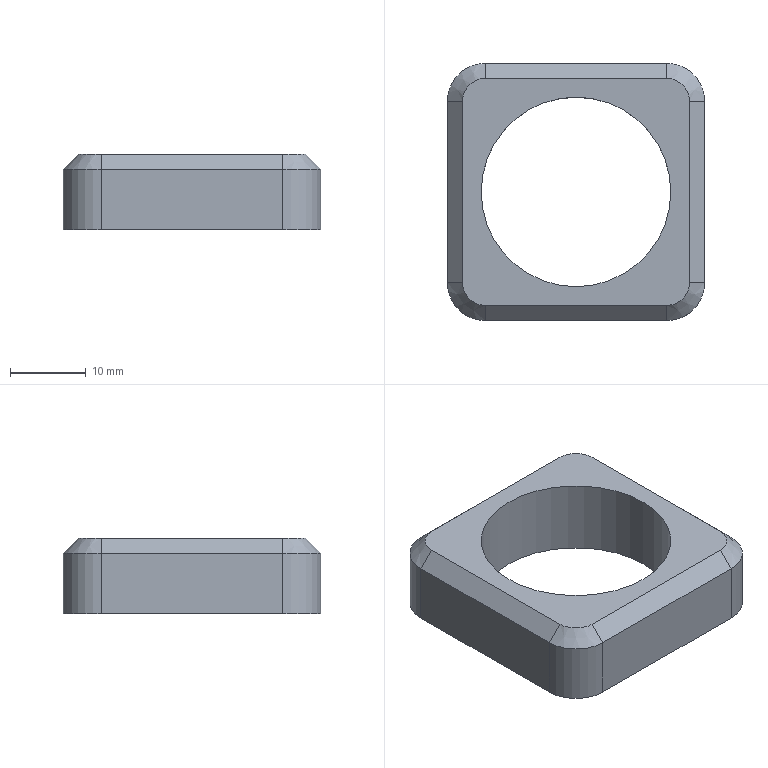Part | STEP file | Sheet34 | 1 solid | 19 faces | box 34 x 34 x 10 mm | volume 6171 mm3 | plane 10 | cylinder 5 | cone 4 | commonest cylinder face diameters 10 x4 25.05 x1
STEP:
#1=CARTESIAN_POINT('',(0.,0.,0.));
#2=DIRECTION('',(0.,0.,1.));
#3=DIRECTION('',(1.,0.,0.));
#4=AXIS2_PLACEMENT_3D('',#1,#2,#3);
#5=CARTESIAN_POINT('',(29.525,-17.,-7.));
#6=VERTEX_POINT('',#5);
#7=CARTESIAN_POINT('',(17.,-17.,-7.));
#8=DIRECTION('',(0.,0.,1.));
#9=DIRECTION('',(-1.,0.,0.));
#10=AXIS2_PLACEMENT_3D('',#7,#8,#9);
#11=CIRCLE('',#10,12.525);
#12=CARTESIAN_POINT('',(17.,-17.,3.));
#13=DIRECTION('',(0.,0.,-1.));
#14=DIRECTION('',(-1.,0.,0.));
#15=AXIS2_PLACEMENT_3D('',#12,#13,#14);
#16=CYLINDRICAL_SURFACE('',#15,12.525);
#17=CARTESIAN_POINT('',(12.566,10.));
#18=DIRECTION('',(-1.,0.));
#19=VECTOR('',#18,1.);
#20=LINE('',#17,#19);
#21=(GEOMETRIC_REPRESENTATION_CONTEXT(2)PARAMETRIC_REPRESENTATION_CONTEXT()REPRESENTATION_CONTEXT('',''));
#22=DEFINITIONAL_REPRESENTATION('',(#20),#21);
#23=PCURVE('',#16,#22);
#24=CARTESIAN_POINT('',(17.,-17.,-7.));
#25=DIRECTION('',(0.,0.,1.));
#26=DIRECTION('',(1.,0.,0.));
#27=AXIS2_PLACEMENT_3D('',#24,#25,#26);
#28=PLANE('',#27);
#29=CARTESIAN_POINT('',(0.,0.));
#30=DIRECTION('',(-1.,0.));
#31=AXIS2_PLACEMENT_2D('',#29,#30);
#32=CIRCLE('',#31,12.525);
#33=(GEOMETRIC_REPRESENTATION_CONTEXT(2)PARAMETRIC_REPRESENTATION_CONTEXT()REPRESENTATION_CONTEXT('',''));
#34=DEFINITIONAL_REPRESENTATION('',(#32),#33);
#35=PCURVE('',#28,#34);
#36=SURFACE_CURVE('',#11,(#23,#35),.PCURVE_S1.);
#37=EDGE_CURVE('',#6,#6,#36,.T.);
#38=ORIENTED_EDGE('',*,*,#37,.T.);
#39=CARTESIAN_POINT('',(29.525,-17.,3.));
#40=VERTEX_POINT('',#39);
#41=CARTESIAN_POINT('',(29.525,-17.,3.));
#42=CARTESIAN_POINT('',(29.525,-17.,-7.));
#43=B_SPLINE_CURVE_WITH_KNOTS('',1,(#41,#42),.UNSPECIFIED.,.F.,.F.,(2,2),(0.,10.),.PIECEWISE_BEZIER_KNOTS.);
#44=CARTESIAN_POINT('',(3.142,0.));
#45=DIRECTION('',(0.,1.));
#46=VECTOR('',#45,1.);
#47=LINE('',#44,#46);
#48=(GEOMETRIC_REPRESENTATION_CONTEXT(2)PARAMETRIC_REPRESENTATION_CONTEXT()REPRESENTATION_CONTEXT('',''));
#49=DEFINITIONAL_REPRESENTATION('',(#47),#48);
#50=PCURVE('',#16,#49);
#51=CARTESIAN_POINT('',(9.425,0.));
#52=DIRECTION('',(0.,1.));
#53=VECTOR('',#52,1.);
#54=LINE('',#51,#53);
#55=(GEOMETRIC_REPRESENTATION_CONTEXT(2)PARAMETRIC_REPRESENTATION_CONTEXT()REPRESENTATION_CONTEXT('',''));
#56=DEFINITIONAL_REPRESENTATION('',(#54),#55);
#57=PCURVE('',#16,#56);
#58=SEAM_CURVE('',#43,(#50,#57),.PCURVE_S1.);
#59=EDGE_CURVE('',#40,#6,#58,.T.);
#60=ORIENTED_EDGE('',*,*,#59,.F.);
#61=CARTESIAN_POINT('',(17.,-17.,3.));
#62=DIRECTION('',(0.,0.,-1.));
#63=DIRECTION('',(-1.,0.,0.));
#64=AXIS2_PLACEMENT_3D('',#61,#62,#63);
#65=CIRCLE('',#64,12.525);
#66=CARTESIAN_POINT('',(0.,0.));
#67=DIRECTION('',(1.,0.));
#68=VECTOR('',#67,1.);
#69=LINE('',#66,#68);
#70=(GEOMETRIC_REPRESENTATION_CONTEXT(2)PARAMETRIC_REPRESENTATION_CONTEXT()REPRESENTATION_CONTEXT('',''));
#71=DEFINITIONAL_REPRESENTATION('',(#69),#70);
#72=PCURVE('',#16,#71);
#73=CARTESIAN_POINT('',(17.,-17.,3.));
#74=DIRECTION('',(0.,0.,1.));
#75=DIRECTION('',(1.,0.,0.));
#76=AXIS2_PLACEMENT_3D('',#73,#74,#75);
#77=PLANE('',#76);
#78=CARTESIAN_POINT('',(-12.525,0.));
#79=CARTESIAN_POINT('',(-12.525,21.694));
#80=CARTESIAN_POINT('',(6.263,10.847));
#81=CARTESIAN_POINT('',(25.05,0.));
#82=CARTESIAN_POINT('',(6.263,-10.847));
#83=CARTESIAN_POINT('',(-12.525,-21.694));
#84=CARTESIAN_POINT('',(-12.525,0.));
#85=(BOUNDED_CURVE()B_SPLINE_CURVE(2,(#78,#79,#80,#81,#82,#83,#84),.UNSPECIFIED.,.T.,.F.)B_SPLINE_CURVE_WITH_KNOTS((1,2,2,2,2,1),(-2.094,0.,2.094,4.189,6.283,8.378),.UNSPECIFIED.)CURVE()GEOMETRIC_REPRESENTATION_ITEM()RATIONAL_B_SPLINE_CURVE((1.,0.5,1.,0.5,1.,0.5,1.))REPRESENTATION_ITEM(''));
#86=(GEOMETRIC_REPRESENTATION_CONTEXT(2)PARAMETRIC_REPRESENTATION_CONTEXT()REPRESENTATION_CONTEXT('',''));
#87=DEFINITIONAL_REPRESENTATION('',(#85),#86);
#88=PCURVE('',#77,#87);
#89=SURFACE_CURVE('',#65,(#72,#88),.PCURVE_S1.);
#90=EDGE_CURVE('',#40,#40,#89,.T.);
#91=ORIENTED_EDGE('',*,*,#90,.T.);
#92=ORIENTED_EDGE('',*,*,#59,.T.);
#93=EDGE_LOOP('',(#38,#60,#91,#92));
#94=FACE_BOUND('',#93,.F.);
#95=ADVANCED_FACE('',(#94),#16,.F.);
#96=CARTESIAN_POINT('',(29.,0.,1.));
#97=VERTEX_POINT('',#96);
#98=CARTESIAN_POINT('',(29.,-2.,3.));
#99=VERTEX_POINT('',#98);
#100=CARTESIAN_POINT('',(29.,0.,1.));
#101=DIRECTION('',(0.,-0.7071,0.7071));
#102=VECTOR('',#101,1.);
#103=LINE('',#100,#102);
#104=CARTESIAN_POINT('',(29.,-5.,2.));
#105=DIRECTION('',(0.,0.,-1.));
#106=DIRECTION('',(1.,0.,0.));
#107=AXIS2_PLACEMENT_3D('',#104,#105,#106);
#108=CONICAL_SURFACE('',#107,4.,0.7854);
#109=CARTESIAN_POINT('',(4.712,1.));
#110=DIRECTION('',(0.,-1.));
#111=VECTOR('',#110,1.);
#112=LINE('',#109,#111);
#113=(GEOMETRIC_REPRESENTATION_CONTEXT(2)PARAMETRIC_REPRESENTATION_CONTEXT()REPRESENTATION_CONTEXT('',''));
#114=DEFINITIONAL_REPRESENTATION('',(#112),#113);
#115=PCURVE('',#108,#114);
#116=CARTESIAN_POINT('',(23.,-1.,2.));
#117=DIRECTION('',(0.,0.7071,0.7071));
#118=DIRECTION('',(1.,0.,0.));
#119=AXIS2_PLACEMENT_3D('',#116,#117,#118);
#120=PLANE('',#119);
#121=CARTESIAN_POINT('',(6.,1.414));
#122=DIRECTION('',(0.,-1.));
#123=VECTOR('',#122,1.);
#124=LINE('',#121,#123);
#125=(GEOMETRIC_REPRESENTATION_CONTEXT(2)PARAMETRIC_REPRESENTATION_CONTEXT()REPRESENTATION_CONTEXT('',''));
#126=DEFINITIONAL_REPRESENTATION('',(#124),#125);
#127=PCURVE('',#120,#126);
#128=SURFACE_CURVE('',#103,(#115,#127),.PCURVE_S1.);
#129=EDGE_CURVE('',#97,#99,#128,.T.);
#130=ORIENTED_EDGE('',*,*,#129,.T.);
#131=CARTESIAN_POINT('',(32.,-5.,3.));
#132=VERTEX_POINT('',#131);
#133=CARTESIAN_POINT('',(29.,-5.,3.));
#134=DIRECTION('',(0.,0.,-1.));
#135=DIRECTION('',(1.,0.,0.));
#136=AXIS2_PLACEMENT_3D('',#133,#134,#135);
#137=CIRCLE('',#136,3.);
#138=CARTESIAN_POINT('',(0.,-1.));
#139=DIRECTION('',(1.,0.));
#140=VECTOR('',#139,1.);
#141=LINE('',#138,#140);
#142=(GEOMETRIC_REPRESENTATION_CONTEXT(2)PARAMETRIC_REPRESENTATION_CONTEXT()REPRESENTATION_CONTEXT('',''));
#143=DEFINITIONAL_REPRESENTATION('',(#141),#142);
#144=PCURVE('',#108,#143);
#145=CARTESIAN_POINT('',(15.,12.));
#146=CARTESIAN_POINT('',(15.,6.804));
#147=CARTESIAN_POINT('',(10.5,9.402));
#148=CARTESIAN_POINT('',(6.,12.));
#149=CARTESIAN_POINT('',(10.5,14.598));
#150=CARTESIAN_POINT('',(15.,17.196));
#151=CARTESIAN_POINT('',(15.,12.));
#152=(BOUNDED_CURVE()B_SPLINE_CURVE(2,(#145,#146,#147,#148,#149,#150,#151),.UNSPECIFIED.,.T.,.F.)B_SPLINE_CURVE_WITH_KNOTS((1,2,2,2,2,1),(-2.094,0.,2.094,4.189,6.283,8.378),.UNSPECIFIED.)CURVE()GEOMETRIC_REPRESENTATION_ITEM()RATIONAL_B_SPLINE_CURVE((1.,0.5,1.,0.5,1.,0.5,1.))REPRESENTATION_ITEM(''));
#153=(GEOMETRIC_REPRESENTATION_CONTEXT(2)PARAMETRIC_REPRESENTATION_CONTEXT()REPRESENTATION_CONTEXT('',''));
#154=DEFINITIONAL_REPRESENTATION('',(#152),#153);
#155=PCURVE('',#77,#154);
#156=SURFACE_CURVE('',#137,(#144,#155),.PCURVE_S1.);
#157=EDGE_CURVE('',#99,#132,#156,.T.);
#158=ORIENTED_EDGE('',*,*,#157,.T.);
#159=CARTESIAN_POINT('',(34.,-5.,1.));
#160=VERTEX_POINT('',#159);
#161=CARTESIAN_POINT('',(32.,-5.,3.));
#162=DIRECTION('',(0.7071,0.,-0.7071));
#163=VECTOR('',#162,1.);
#164=LINE('',#161,#163);
#165=CARTESIAN_POINT('',(6.283,-1.));
#166=DIRECTION('',(0.,1.));
#167=VECTOR('',#166,1.);
#168=LINE('',#165,#167);
#169=(GEOMETRIC_REPRESENTATION_CONTEXT(2)PARAMETRIC_REPRESENTATION_CONTEXT()REPRESENTATION_CONTEXT('',''));
#170=DEFINITIONAL_REPRESENTATION('',(#168),#169);
#171=PCURVE('',#108,#170);
#172=CARTESIAN_POINT('',(33.,-23.,2.));
#173=DIRECTION('',(0.7071,0.,0.7071));
#174=DIRECTION('',(0.7071,0.,-0.7071));
#175=AXIS2_PLACEMENT_3D('',#172,#173,#174);
#176=PLANE('',#175);
#177=CARTESIAN_POINT('',(-1.414,18.));
#178=DIRECTION('',(1.,0.));
#179=VECTOR('',#178,1.);
#180=LINE('',#177,#179);
#181=(GEOMETRIC_REPRESENTATION_CONTEXT(2)PARAMETRIC_REPRESENTATION_CONTEXT()REPRESENTATION_CONTEXT('',''));
#182=DEFINITIONAL_REPRESENTATION('',(#180),#181);
#183=PCURVE('',#176,#182);
#184=SURFACE_CURVE('',#164,(#171,#183),.PCURVE_S1.);
#185=EDGE_CURVE('',#132,#160,#184,.T.);
#186=ORIENTED_EDGE('',*,*,#185,.T.);
#187=CARTESIAN_POINT('',(29.,-5.,1.));
#188=DIRECTION('',(0.,0.,1.));
#189=DIRECTION('',(1.,0.,0.));
#190=AXIS2_PLACEMENT_3D('',#187,#188,#189);
#191=CIRCLE('',#190,5.);
#192=CARTESIAN_POINT('',(6.283,1.));
#193=DIRECTION('',(-1.,0.));
#194=VECTOR('',#193,1.);
#195=LINE('',#192,#194);
#196=(GEOMETRIC_REPRESENTATION_CONTEXT(2)PARAMETRIC_REPRESENTATION_CONTEXT()REPRESENTATION_CONTEXT('',''));
#197=DEFINITIONAL_REPRESENTATION('',(#195),#196);
#198=PCURVE('',#108,#197);
#199=CARTESIAN_POINT('',(29.,-5.,0.));
#200=DIRECTION('',(0.,0.,1.));
#201=DIRECTION('',(-1.,0.,0.));
#202=AXIS2_PLACEMENT_3D('',#199,#200,#201);
#203=CYLINDRICAL_SURFACE('',#202,5.);
#204=CARTESIAN_POINT('',(3.142,1.));
#205=DIRECTION('',(1.,0.));
#206=VECTOR('',#205,1.);
#207=LINE('',#204,#206);
#208=(GEOMETRIC_REPRESENTATION_CONTEXT(2)PARAMETRIC_REPRESENTATION_CONTEXT()REPRESENTATION_CONTEXT('',''));
#209=DEFINITIONAL_REPRESENTATION('',(#207),#208);
#210=PCURVE('',#203,#209);
#211=SURFACE_CURVE('',#191,(#198,#210),.PCURVE_S1.);
#212=EDGE_CURVE('',#160,#97,#211,.T.);
#213=ORIENTED_EDGE('',*,*,#212,.T.);
#214=EDGE_LOOP('',(#130,#158,#186,#213));
#215=FACE_BOUND('',#214,.T.);
#216=ADVANCED_FACE('',(#215),#108,.T.);
#217=CARTESIAN_POINT('',(5.,0.,1.));
#218=VERTEX_POINT('',#217);
#219=CARTESIAN_POINT('',(5.,-2.,3.));
#220=VERTEX_POINT('',#219);
#221=CARTESIAN_POINT('',(5.,0.,1.));
#222=DIRECTION('',(0.,-0.7071,0.7071));
#223=VECTOR('',#222,1.);
#224=LINE('',#221,#223);
#225=CARTESIAN_POINT('',(-18.,1.414));
#226=DIRECTION('',(0.,-1.));
#227=VECTOR('',#226,1.);
#228=LINE('',#225,#227);
#229=(GEOMETRIC_REPRESENTATION_CONTEXT(2)PARAMETRIC_REPRESENTATION_CONTEXT()REPRESENTATION_CONTEXT('',''));
#230=DEFINITIONAL_REPRESENTATION('',(#228),#229);
#231=PCURVE('',#120,#230);
#232=CARTESIAN_POINT('',(5.,-5.,2.));
#233=DIRECTION('',(0.,0.,-1.));
#234=DIRECTION('',(0.,1.,0.));
#235=AXIS2_PLACEMENT_3D('',#232,#233,#234);
#236=CONICAL_SURFACE('',#235,4.,0.7854);
#237=CARTESIAN_POINT('',(6.283,1.));
#238=DIRECTION('',(0.,-1.));
#239=VECTOR('',#238,1.);
#240=LINE('',#237,#239);
#241=(GEOMETRIC_REPRESENTATION_CONTEXT(2)PARAMETRIC_REPRESENTATION_CONTEXT()REPRESENTATION_CONTEXT('',''));
#242=DEFINITIONAL_REPRESENTATION('',(#240),#241);
#243=PCURVE('',#236,#242);
#244=SURFACE_CURVE('',#224,(#231,#243),.PCURVE_S1.);
#245=EDGE_CURVE('',#218,#220,#244,.T.);
#246=ORIENTED_EDGE('',*,*,#245,.T.);
#247=CARTESIAN_POINT('',(23.,-2.,3.));
#248=DIRECTION('',(1.,0.,0.));
#249=VECTOR('',#248,1.);
#250=LINE('',#247,#249);
#251=CARTESIAN_POINT('',(0.,-1.414));
#252=DIRECTION('',(1.,0.));
#253=VECTOR('',#252,1.);
#254=LINE('',#251,#253);
#255=(GEOMETRIC_REPRESENTATION_CONTEXT(2)PARAMETRIC_REPRESENTATION_CONTEXT()REPRESENTATION_CONTEXT('',''));
#256=DEFINITIONAL_REPRESENTATION('',(#254),#255);
#257=PCURVE('',#120,#256);
#258=CARTESIAN_POINT('',(6.,15.));
#259=DIRECTION('',(1.,0.));
#260=VECTOR('',#259,1.);
#261=LINE('',#258,#260);
#262=(GEOMETRIC_REPRESENTATION_CONTEXT(2)PARAMETRIC_REPRESENTATION_CONTEXT()REPRESENTATION_CONTEXT('',''));
#263=DEFINITIONAL_REPRESENTATION('',(#261),#262);
#264=PCURVE('',#77,#263);
#265=SURFACE_CURVE('',#250,(#257,#264),.PCURVE_S1.);
#266=EDGE_CURVE('',#220,#99,#265,.T.);
#267=ORIENTED_EDGE('',*,*,#266,.T.);
#268=ORIENTED_EDGE('',*,*,#129,.F.);
#269=CARTESIAN_POINT('',(23.,0.,1.));
#270=DIRECTION('',(-1.,0.,0.));
#271=VECTOR('',#270,1.);
#272=LINE('',#269,#271);
#273=CARTESIAN_POINT('',(0.,1.414));
#274=DIRECTION('',(-1.,0.));
#275=VECTOR('',#274,1.);
#276=LINE('',#273,#275);
#277=(GEOMETRIC_REPRESENTATION_CONTEXT(2)PARAMETRIC_REPRESENTATION_CONTEXT()REPRESENTATION_CONTEXT('',''));
#278=DEFINITIONAL_REPRESENTATION('',(#276),#277);
#279=PCURVE('',#120,#278);
#280=CARTESIAN_POINT('',(29.,0.,0.));
#281=DIRECTION('',(0.,1.,0.));
#282=DIRECTION('',(-1.,0.,0.));
#283=AXIS2_PLACEMENT_3D('',#280,#281,#282);
#284=PLANE('',#283);
#285=CARTESIAN_POINT('',(6.,1.));
#286=DIRECTION('',(1.,0.));
#287=VECTOR('',#286,1.);
#288=LINE('',#285,#287);
#289=(GEOMETRIC_REPRESENTATION_CONTEXT(2)PARAMETRIC_REPRESENTATION_CONTEXT()REPRESENTATION_CONTEXT('',''));
#290=DEFINITIONAL_REPRESENTATION('',(#288),#289);
#291=PCURVE('',#284,#290);
#292=SURFACE_CURVE('',#272,(#279,#291),.PCURVE_S1.);
#293=EDGE_CURVE('',#97,#218,#292,.T.);
#294=ORIENTED_EDGE('',*,*,#293,.T.);
#295=EDGE_LOOP('',(#246,#267,#268,#294));
#296=FACE_BOUND('',#295,.T.);
#297=ADVANCED_FACE('',(#296),#120,.T.);
#298=CARTESIAN_POINT('',(0.,-5.,1.));
#299=VERTEX_POINT('',#298);
#300=CARTESIAN_POINT('',(2.,-5.,3.));
#301=VERTEX_POINT('',#300);
#302=CARTESIAN_POINT('',(0.,-5.,1.));
#303=DIRECTION('',(0.7071,0.,0.7071));
#304=VECTOR('',#303,1.);
#305=LINE('',#302,#304);
#306=CARTESIAN_POINT('',(4.712,1.));
#307=DIRECTION('',(0.,-1.));
#308=VECTOR('',#307,1.);
#309=LINE('',#306,#308);
#310=(GEOMETRIC_REPRESENTATION_CONTEXT(2)PARAMETRIC_REPRESENTATION_CONTEXT()REPRESENTATION_CONTEXT('',''));
#311=DEFINITIONAL_REPRESENTATION('',(#309),#310);
#312=PCURVE('',#236,#311);
#313=CARTESIAN_POINT('',(1.,-11.,2.));
#314=DIRECTION('',(-0.7071,0.,0.7071));
#315=DIRECTION('',(0.7071,0.,0.7071));
#316=AXIS2_PLACEMENT_3D('',#313,#314,#315);
#317=PLANE('',#316);
#318=CARTESIAN_POINT('',(-1.414,6.));
#319=DIRECTION('',(1.,0.));
#320=VECTOR('',#319,1.);
#321=LINE('',#318,#320);
#322=(GEOMETRIC_REPRESENTATION_CONTEXT(2)PARAMETRIC_REPRESENTATION_CONTEXT()REPRESENTATION_CONTEXT('',''));
#323=DEFINITIONAL_REPRESENTATION('',(#321),#322);
#324=PCURVE('',#317,#323);
#325=SURFACE_CURVE('',#305,(#312,#324),.PCURVE_S1.);
#326=EDGE_CURVE('',#299,#301,#325,.T.);
#327=ORIENTED_EDGE('',*,*,#326,.T.);
#328=CARTESIAN_POINT('',(5.,-5.,3.));
#329=DIRECTION('',(0.,0.,-1.));
#330=DIRECTION('',(0.,1.,0.));
#331=AXIS2_PLACEMENT_3D('',#328,#329,#330);
#332=CIRCLE('',#331,3.);
#333=CARTESIAN_POINT('',(0.,-1.));
#334=DIRECTION('',(1.,0.));
#335=VECTOR('',#334,1.);
#336=LINE('',#333,#335);
#337=(GEOMETRIC_REPRESENTATION_CONTEXT(2)PARAMETRIC_REPRESENTATION_CONTEXT()REPRESENTATION_CONTEXT('',''));
#338=DEFINITIONAL_REPRESENTATION('',(#336),#337);
#339=PCURVE('',#236,#338);
#340=CARTESIAN_POINT('',(-12.,15.));
#341=CARTESIAN_POINT('',(-6.804,15.));
#342=CARTESIAN_POINT('',(-9.402,10.5));
#343=CARTESIAN_POINT('',(-12.,6.));
#344=CARTESIAN_POINT('',(-14.598,10.5));
#345=CARTESIAN_POINT('',(-17.196,15.));
#346=CARTESIAN_POINT('',(-12.,15.));
#347=(BOUNDED_CURVE()B_SPLINE_CURVE(2,(#340,#341,#342,#343,#344,#345,#346),.UNSPECIFIED.,.T.,.F.)B_SPLINE_CURVE_WITH_KNOTS((1,2,2,2,2,1),(-2.094,0.,2.094,4.189,6.283,8.378),.UNSPECIFIED.)CURVE()GEOMETRIC_REPRESENTATION_ITEM()RATIONAL_B_SPLINE_CURVE((1.,0.5,1.,0.5,1.,0.5,1.))REPRESENTATION_ITEM(''));
#348=(GEOMETRIC_REPRESENTATION_CONTEXT(2)PARAMETRIC_REPRESENTATION_CONTEXT()REPRESENTATION_CONTEXT('',''));
#349=DEFINITIONAL_REPRESENTATION('',(#347),#348);
#350=PCURVE('',#77,#349);
#351=SURFACE_CURVE('',#332,(#339,#350),.PCURVE_S1.);
#352=EDGE_CURVE('',#301,#220,#351,.T.);
#353=ORIENTED_EDGE('',*,*,#352,.T.);
#354=ORIENTED_EDGE('',*,*,#245,.F.);
#355=CARTESIAN_POINT('',(5.,-5.,1.));
#356=DIRECTION('',(0.,0.,1.));
#357=DIRECTION('',(0.,1.,0.));
#358=AXIS2_PLACEMENT_3D('',#355,#356,#357);
#359=CIRCLE('',#358,5.);
#360=CARTESIAN_POINT('',(6.283,1.));
#361=DIRECTION('',(-1.,0.));
#362=VECTOR('',#361,1.);
#363=LINE('',#360,#362);
#364=(GEOMETRIC_REPRESENTATION_CONTEXT(2)PARAMETRIC_REPRESENTATION_CONTEXT()REPRESENTATION_CONTEXT('',''));
#365=DEFINITIONAL_REPRESENTATION('',(#363),#364);
#366=PCURVE('',#236,#365);
#367=CARTESIAN_POINT('',(5.,-5.,0.));
#368=DIRECTION('',(0.,0.,1.));
#369=DIRECTION('',(0.,-1.,0.));
#370=AXIS2_PLACEMENT_3D('',#367,#368,#369);
#371=CYLINDRICAL_SURFACE('',#370,5.);
#372=CARTESIAN_POINT('',(3.142,1.));
#373=DIRECTION('',(1.,0.));
#374=VECTOR('',#373,1.);
#375=LINE('',#372,#374);
#376=(GEOMETRIC_REPRESENTATION_CONTEXT(2)PARAMETRIC_REPRESENTATION_CONTEXT()REPRESENTATION_CONTEXT('',''));
#377=DEFINITIONAL_REPRESENTATION('',(#375),#376);
#378=PCURVE('',#371,#377);
#379=SURFACE_CURVE('',#359,(#366,#378),.PCURVE_S1.);
#380=EDGE_CURVE('',#218,#299,#379,.T.);
#381=ORIENTED_EDGE('',*,*,#380,.T.);
#382=EDGE_LOOP('',(#327,#353,#354,#381));
#383=FACE_BOUND('',#382,.T.);
#384=ADVANCED_FACE('',(#383),#236,.T.);
#385=CARTESIAN_POINT('',(0.,-29.,1.));
#386=VERTEX_POINT('',#385);
#387=CARTESIAN_POINT('',(2.,-29.,3.));
#388=VERTEX_POINT('',#387);
#389=CARTESIAN_POINT('',(0.,-29.,1.));
#390=DIRECTION('',(0.7071,0.,0.7071));
#391=VECTOR('',#390,1.);
#392=LINE('',#389,#391);
#393=CARTESIAN_POINT('',(-1.414,-18.));
#394=DIRECTION('',(1.,0.));
#395=VECTOR('',#394,1.);
#396=LINE('',#393,#395);
#397=(GEOMETRIC_REPRESENTATION_CONTEXT(2)PARAMETRIC_REPRESENTATION_CONTEXT()REPRESENTATION_CONTEXT('',''));
#398=DEFINITIONAL_REPRESENTATION('',(#396),#397);
#399=PCURVE('',#317,#398);
#400=CARTESIAN_POINT('',(5.,-29.,2.));
#401=DIRECTION('',(0.,0.,-1.));
#402=DIRECTION('',(-1.,0.,0.));
#403=AXIS2_PLACEMENT_3D('',#400,#401,#402);
#404=CONICAL_SURFACE('',#403,4.,0.7854);
#405=CARTESIAN_POINT('',(6.283,1.));
#406=DIRECTION('',(0.,-1.));
#407=VECTOR('',#406,1.);
#408=LINE('',#405,#407);
#409=(GEOMETRIC_REPRESENTATION_CONTEXT(2)PARAMETRIC_REPRESENTATION_CONTEXT()REPRESENTATION_CONTEXT('',''));
#410=DEFINITIONAL_REPRESENTATION('',(#408),#409);
#411=PCURVE('',#404,#410);
#412=SURFACE_CURVE('',#392,(#399,#411),.PCURVE_S1.);
#413=EDGE_CURVE('',#386,#388,#412,.T.);
#414=ORIENTED_EDGE('',*,*,#413,.T.);
#415=CARTESIAN_POINT('',(2.,-11.,3.));
#416=DIRECTION('',(0.,1.,0.));
#417=VECTOR('',#416,1.);
#418=LINE('',#415,#417);
#419=CARTESIAN_POINT('',(1.414,0.));
#420=DIRECTION('',(0.,1.));
#421=VECTOR('',#420,1.);
#422=LINE('',#419,#421);
#423=(GEOMETRIC_REPRESENTATION_CONTEXT(2)PARAMETRIC_REPRESENTATION_CONTEXT()REPRESENTATION_CONTEXT('',''));
#424=DEFINITIONAL_REPRESENTATION('',(#422),#423);
#425=PCURVE('',#317,#424);
#426=CARTESIAN_POINT('',(-15.,6.));
#427=DIRECTION('',(0.,1.));
#428=VECTOR('',#427,1.);
#429=LINE('',#426,#428);
#430=(GEOMETRIC_REPRESENTATION_CONTEXT(2)PARAMETRIC_REPRESENTATION_CONTEXT()REPRESENTATION_CONTEXT('',''));
#431=DEFINITIONAL_REPRESENTATION('',(#429),#430);
#432=PCURVE('',#77,#431);
#433=SURFACE_CURVE('',#418,(#425,#432),.PCURVE_S1.);
#434=EDGE_CURVE('',#388,#301,#433,.T.);
#435=ORIENTED_EDGE('',*,*,#434,.T.);
#436=ORIENTED_EDGE('',*,*,#326,.F.);
#437=CARTESIAN_POINT('',(0.,-11.,1.));
#438=DIRECTION('',(0.,-1.,0.));
#439=VECTOR('',#438,1.);
#440=LINE('',#437,#439);
#441=CARTESIAN_POINT('',(-1.414,0.));
#442=DIRECTION('',(0.,-1.));
#443=VECTOR('',#442,1.);
#444=LINE('',#441,#443);
#445=(GEOMETRIC_REPRESENTATION_CONTEXT(2)PARAMETRIC_REPRESENTATION_CONTEXT()REPRESENTATION_CONTEXT('',''));
#446=DEFINITIONAL_REPRESENTATION('',(#444),#445);
#447=PCURVE('',#317,#446);
#448=CARTESIAN_POINT('',(0.,-5.,0.));
#449=DIRECTION('',(-1.,0.,0.));
#450=DIRECTION('',(0.,-1.,0.));
#451=AXIS2_PLACEMENT_3D('',#448,#449,#450);
#452=PLANE('',#451);
#453=CARTESIAN_POINT('',(6.,1.));
#454=DIRECTION('',(1.,0.));
#455=VECTOR('',#454,1.);
#456=LINE('',#453,#455);
#457=(GEOMETRIC_REPRESENTATION_CONTEXT(2)PARAMETRIC_REPRESENTATION_CONTEXT()REPRESENTATION_CONTEXT('',''));
#458=DEFINITIONAL_REPRESENTATION('',(#456),#457);
#459=PCURVE('',#452,#458);
#460=SURFACE_CURVE('',#440,(#447,#459),.PCURVE_S1.);
#461=EDGE_CURVE('',#299,#386,#460,.T.);
#462=ORIENTED_EDGE('',*,*,#461,.T.);
#463=EDGE_LOOP('',(#414,#435,#436,#462));
#464=FACE_BOUND('',#463,.T.);
#465=ADVANCED_FACE('',(#464),#317,.T.);
#466=CARTESIAN_POINT('',(5.,-34.,1.));
#467=VERTEX_POINT('',#466);
#468=CARTESIAN_POINT('',(5.,-32.,3.));
#469=VERTEX_POINT('',#468);
#470=CARTESIAN_POINT('',(5.,-34.,1.));
#471=DIRECTION('',(0.,0.7071,0.7071));
#472=VECTOR('',#471,1.);
#473=LINE('',#470,#472);
#474=CARTESIAN_POINT('',(4.712,1.));
#475=DIRECTION('',(0.,-1.));
#476=VECTOR('',#475,1.);
#477=LINE('',#474,#476);
#478=(GEOMETRIC_REPRESENTATION_CONTEXT(2)PARAMETRIC_REPRESENTATION_CONTEXT()REPRESENTATION_CONTEXT('',''));
#479=DEFINITIONAL_REPRESENTATION('',(#477),#478);
#480=PCURVE('',#404,#479);
#481=CARTESIAN_POINT('',(11.,-33.,2.));
#482=DIRECTION('',(0.,-0.7071,0.7071));
#483=DIRECTION('',(1.,0.,0.));
#484=AXIS2_PLACEMENT_3D('',#481,#482,#483);
#485=PLANE('',#484);
#486=CARTESIAN_POINT('',(-6.,-1.414));
#487=DIRECTION('',(0.,1.));
#488=VECTOR('',#487,1.);
#489=LINE('',#486,#488);
#490=(GEOMETRIC_REPRESENTATION_CONTEXT(2)PARAMETRIC_REPRESENTATION_CONTEXT()REPRESENTATION_CONTEXT('',''));
#491=DEFINITIONAL_REPRESENTATION('',(#489),#490);
#492=PCURVE('',#485,#491);
#493=SURFACE_CURVE('',#473,(#480,#492),.PCURVE_S1.);
#494=EDGE_CURVE('',#467,#469,#493,.T.);
#495=ORIENTED_EDGE('',*,*,#494,.T.);
#496=CARTESIAN_POINT('',(5.,-29.,3.));
#497=DIRECTION('',(0.,0.,-1.));
#498=DIRECTION('',(-1.,0.,0.));
#499=AXIS2_PLACEMENT_3D('',#496,#497,#498);
#500=CIRCLE('',#499,3.);
#501=CARTESIAN_POINT('',(0.,-1.));
#502=DIRECTION('',(1.,0.));
#503=VECTOR('',#502,1.);
#504=LINE('',#501,#503);
#505=(GEOMETRIC_REPRESENTATION_CONTEXT(2)PARAMETRIC_REPRESENTATION_CONTEXT()REPRESENTATION_CONTEXT('',''));
#506=DEFINITIONAL_REPRESENTATION('',(#504),#505);
#507=PCURVE('',#404,#506);
#508=CARTESIAN_POINT('',(-15.,-12.));
#509=CARTESIAN_POINT('',(-15.,-6.804));
#510=CARTESIAN_POINT('',(-10.5,-9.402));
#511=CARTESIAN_POINT('',(-6.,-12.));
#512=CARTESIAN_POINT('',(-10.5,-14.598));
#513=CARTESIAN_POINT('',(-15.,-17.196));
#514=CARTESIAN_POINT('',(-15.,-12.));
#515=(BOUNDED_CURVE()B_SPLINE_CURVE(2,(#508,#509,#510,#511,#512,#513,#514),.UNSPECIFIED.,.T.,.F.)B_SPLINE_CURVE_WITH_KNOTS((1,2,2,2,2,1),(-2.094,0.,2.094,4.189,6.283,8.378),.UNSPECIFIED.)CURVE()GEOMETRIC_REPRESENTATION_ITEM()RATIONAL_B_SPLINE_CURVE((1.,0.5,1.,0.5,1.,0.5,1.))REPRESENTATION_ITEM(''));
#516=(GEOMETRIC_REPRESENTATION_CONTEXT(2)PARAMETRIC_REPRESENTATION_CONTEXT()REPRESENTATION_CONTEXT('',''));
#517=DEFINITIONAL_REPRESENTATION('',(#515),#516);
#518=PCURVE('',#77,#517);
#519=SURFACE_CURVE('',#500,(#507,#518),.PCURVE_S1.);
#520=EDGE_CURVE('',#469,#388,#519,.T.);
#521=ORIENTED_EDGE('',*,*,#520,.T.);
#522=ORIENTED_EDGE('',*,*,#413,.F.);
#523=CARTESIAN_POINT('',(5.,-29.,1.));
#524=DIRECTION('',(0.,0.,1.));
#525=DIRECTION('',(-1.,0.,0.));
#526=AXIS2_PLACEMENT_3D('',#523,#524,#525);
#527=CIRCLE('',#526,5.);
#528=CARTESIAN_POINT('',(6.283,1.));
#529=DIRECTION('',(-1.,0.));
#530=VECTOR('',#529,1.);
#531=LINE('',#528,#530);
#532=(GEOMETRIC_REPRESENTATION_CONTEXT(2)PARAMETRIC_REPRESENTATION_CONTEXT()REPRESENTATION_CONTEXT('',''));
#533=DEFINITIONAL_REPRESENTATION('',(#531),#532);
#534=PCURVE('',#404,#533);
#535=CARTESIAN_POINT('',(5.,-29.,0.));
#536=DIRECTION('',(0.,0.,1.));
#537=DIRECTION('',(1.,0.,0.));
#538=AXIS2_PLACEMENT_3D('',#535,#536,#537);
#539=CYLINDRICAL_SURFACE('',#538,5.);
#540=CARTESIAN_POINT('',(3.142,1.));
#541=DIRECTION('',(1.,0.));
#542=VECTOR('',#541,1.);
#543=LINE('',#540,#542);
#544=(GEOMETRIC_REPRESENTATION_CONTEXT(2)PARAMETRIC_REPRESENTATION_CONTEXT()REPRESENTATION_CONTEXT('',''));
#545=DEFINITIONAL_REPRESENTATION('',(#543),#544);
#546=PCURVE('',#539,#545);
#547=SURFACE_CURVE('',#527,(#534,#546),.PCURVE_S1.);
#548=EDGE_CURVE('',#386,#467,#547,.T.);
#549=ORIENTED_EDGE('',*,*,#548,.T.);
#550=EDGE_LOOP('',(#495,#521,#522,#549));
#551=FACE_BOUND('',#550,.T.);
#552=ADVANCED_FACE('',(#551),#404,.T.);
#553=CARTESIAN_POINT('',(29.,-34.,1.));
#554=VERTEX_POINT('',#553);
#555=CARTESIAN_POINT('',(29.,-32.,3.));
#556=VERTEX_POINT('',#555);
#557=CARTESIAN_POINT('',(29.,-34.,1.));
#558=DIRECTION('',(0.,0.7071,0.7071));
#559=VECTOR('',#558,1.);
#560=LINE('',#557,#559);
#561=CARTESIAN_POINT('',(18.,-1.414));
#562=DIRECTION('',(0.,1.));
#563=VECTOR('',#562,1.);
#564=LINE('',#561,#563);
#565=(GEOMETRIC_REPRESENTATION_CONTEXT(2)PARAMETRIC_REPRESENTATION_CONTEXT()REPRESENTATION_CONTEXT('',''));
#566=DEFINITIONAL_REPRESENTATION('',(#564),#565);
#567=PCURVE('',#485,#566);
#568=CARTESIAN_POINT('',(29.,-29.,2.));
#569=DIRECTION('',(0.,0.,-1.));
#570=DIRECTION('',(0.,-1.,0.));
#571=AXIS2_PLACEMENT_3D('',#568,#569,#570);
#572=CONICAL_SURFACE('',#571,4.,0.7854);
#573=CARTESIAN_POINT('',(6.283,1.));
#574=DIRECTION('',(0.,-1.));
#575=VECTOR('',#574,1.);
#576=LINE('',#573,#575);
#577=(GEOMETRIC_REPRESENTATION_CONTEXT(2)PARAMETRIC_REPRESENTATION_CONTEXT()REPRESENTATION_CONTEXT('',''));
#578=DEFINITIONAL_REPRESENTATION('',(#576),#577);
#579=PCURVE('',#572,#578);
#580=SURFACE_CURVE('',#560,(#567,#579),.PCURVE_S1.);
#581=EDGE_CURVE('',#554,#556,#580,.T.);
#582=ORIENTED_EDGE('',*,*,#581,.T.);
#583=CARTESIAN_POINT('',(11.,-32.,3.));
#584=DIRECTION('',(-1.,0.,0.));
#585=VECTOR('',#584,1.);
#586=LINE('',#583,#585);
#587=CARTESIAN_POINT('',(0.,1.414));
#588=DIRECTION('',(-1.,0.));
#589=VECTOR('',#588,1.);
#590=LINE('',#587,#589);
#591=(GEOMETRIC_REPRESENTATION_CONTEXT(2)PARAMETRIC_REPRESENTATION_CONTEXT()REPRESENTATION_CONTEXT('',''));
#592=DEFINITIONAL_REPRESENTATION('',(#590),#591);
#593=PCURVE('',#485,#592);
#594=CARTESIAN_POINT('',(-6.,-15.));
#595=DIRECTION('',(-1.,0.));
#596=VECTOR('',#595,1.);
#597=LINE('',#594,#596);
#598=(GEOMETRIC_REPRESENTATION_CONTEXT(2)PARAMETRIC_REPRESENTATION_CONTEXT()REPRESENTATION_CONTEXT('',''));
#599=DEFINITIONAL_REPRESENTATION('',(#597),#598);
#600=PCURVE('',#77,#599);
#601=SURFACE_CURVE('',#586,(#593,#600),.PCURVE_S1.);
#602=EDGE_CURVE('',#556,#469,#601,.T.);
#603=ORIENTED_EDGE('',*,*,#602,.T.);
#604=ORIENTED_EDGE('',*,*,#494,.F.);
#605=CARTESIAN_POINT('',(11.,-34.,1.));
#606=DIRECTION('',(1.,0.,0.));
#607=VECTOR('',#606,1.);
#608=LINE('',#605,#607);
#609=CARTESIAN_POINT('',(0.,-1.414));
#610=DIRECTION('',(1.,0.));
#611=VECTOR('',#610,1.);
#612=LINE('',#609,#611);
#613=(GEOMETRIC_REPRESENTATION_CONTEXT(2)PARAMETRIC_REPRESENTATION_CONTEXT()REPRESENTATION_CONTEXT('',''));
#614=DEFINITIONAL_REPRESENTATION('',(#612),#613);
#615=PCURVE('',#485,#614);
#616=CARTESIAN_POINT('',(5.,-34.,0.));
#617=DIRECTION('',(0.,-1.,0.));
#618=DIRECTION('',(1.,0.,0.));
#619=AXIS2_PLACEMENT_3D('',#616,#617,#618);
#620=PLANE('',#619);
#621=CARTESIAN_POINT('',(6.,1.));
#622=DIRECTION('',(1.,0.));
#623=VECTOR('',#622,1.);
#624=LINE('',#621,#623);
#625=(GEOMETRIC_REPRESENTATION_CONTEXT(2)PARAMETRIC_REPRESENTATION_CONTEXT()REPRESENTATION_CONTEXT('',''));
#626=DEFINITIONAL_REPRESENTATION('',(#624),#625);
#627=PCURVE('',#620,#626);
#628=SURFACE_CURVE('',#608,(#615,#627),.PCURVE_S1.);
#629=EDGE_CURVE('',#467,#554,#628,.T.);
#630=ORIENTED_EDGE('',*,*,#629,.T.);
#631=EDGE_LOOP('',(#582,#603,#604,#630));
#632=FACE_BOUND('',#631,.T.);
#633=ADVANCED_FACE('',(#632),#485,.T.);
#634=CARTESIAN_POINT('',(34.,-29.,1.));
#635=VERTEX_POINT('',#634);
#636=CARTESIAN_POINT('',(32.,-29.,3.));
#637=VERTEX_POINT('',#636);
#638=CARTESIAN_POINT('',(34.,-29.,1.));
#639=DIRECTION('',(-0.7071,0.,0.7071));
#640=VECTOR('',#639,1.);
#641=LINE('',#638,#640);
#642=CARTESIAN_POINT('',(4.712,1.));
#643=DIRECTION('',(0.,-1.));
#644=VECTOR('',#643,1.);
#645=LINE('',#642,#644);
#646=(GEOMETRIC_REPRESENTATION_CONTEXT(2)PARAMETRIC_REPRESENTATION_CONTEXT()REPRESENTATION_CONTEXT('',''));
#647=DEFINITIONAL_REPRESENTATION('',(#645),#646);
#648=PCURVE('',#572,#647);
#649=CARTESIAN_POINT('',(1.414,-6.));
#650=DIRECTION('',(-1.,0.));
#651=VECTOR('',#650,1.);
#652=LINE('',#649,#651);
#653=(GEOMETRIC_REPRESENTATION_CONTEXT(2)PARAMETRIC_REPRESENTATION_CONTEXT()REPRESENTATION_CONTEXT('',''));
#654=DEFINITIONAL_REPRESENTATION('',(#652),#653);
#655=PCURVE('',#176,#654);
#656=SURFACE_CURVE('',#641,(#648,#655),.PCURVE_S1.);
#657=EDGE_CURVE('',#635,#637,#656,.T.);
#658=ORIENTED_EDGE('',*,*,#657,.T.);
#659=CARTESIAN_POINT('',(29.,-29.,3.));
#660=DIRECTION('',(0.,0.,-1.));
#661=DIRECTION('',(0.,-1.,0.));
#662=AXIS2_PLACEMENT_3D('',#659,#660,#661);
#663=CIRCLE('',#662,3.);
#664=CARTESIAN_POINT('',(0.,-1.));
#665=DIRECTION('',(1.,0.));
#666=VECTOR('',#665,1.);
#667=LINE('',#664,#666);
#668=(GEOMETRIC_REPRESENTATION_CONTEXT(2)PARAMETRIC_REPRESENTATION_CONTEXT()REPRESENTATION_CONTEXT('',''));
#669=DEFINITIONAL_REPRESENTATION('',(#667),#668);
#670=PCURVE('',#572,#669);
#671=CARTESIAN_POINT('',(12.,-15.));
#672=CARTESIAN_POINT('',(6.804,-15.));
#673=CARTESIAN_POINT('',(9.402,-10.5));
#674=CARTESIAN_POINT('',(12.,-6.));
#675=CARTESIAN_POINT('',(14.598,-10.5));
#676=CARTESIAN_POINT('',(17.196,-15.));
#677=CARTESIAN_POINT('',(12.,-15.));
#678=(BOUNDED_CURVE()B_SPLINE_CURVE(2,(#671,#672,#673,#674,#675,#676,#677),.UNSPECIFIED.,.T.,.F.)B_SPLINE_CURVE_WITH_KNOTS((1,2,2,2,2,1),(-2.094,0.,2.094,4.189,6.283,8.378),.UNSPECIFIED.)CURVE()GEOMETRIC_REPRESENTATION_ITEM()RATIONAL_B_SPLINE_CURVE((1.,0.5,1.,0.5,1.,0.5,1.))REPRESENTATION_ITEM(''));
#679=(GEOMETRIC_REPRESENTATION_CONTEXT(2)PARAMETRIC_REPRESENTATION_CONTEXT()REPRESENTATION_CONTEXT('',''));
#680=DEFINITIONAL_REPRESENTATION('',(#678),#679);
#681=PCURVE('',#77,#680);
#682=SURFACE_CURVE('',#663,(#670,#681),.PCURVE_S1.);
#683=EDGE_CURVE('',#637,#556,#682,.T.);
#684=ORIENTED_EDGE('',*,*,#683,.T.);
#685=ORIENTED_EDGE('',*,*,#581,.F.);
#686=CARTESIAN_POINT('',(29.,-29.,1.));
#687=DIRECTION('',(0.,0.,1.));
#688=DIRECTION('',(0.,-1.,0.));
#689=AXIS2_PLACEMENT_3D('',#686,#687,#688);
#690=CIRCLE('',#689,5.);
#691=CARTESIAN_POINT('',(6.283,1.));
#692=DIRECTION('',(-1.,0.));
#693=VECTOR('',#692,1.);
#694=LINE('',#691,#693);
#695=(GEOMETRIC_REPRESENTATION_CONTEXT(2)PARAMETRIC_REPRESENTATION_CONTEXT()REPRESENTATION_CONTEXT('',''));
#696=DEFINITIONAL_REPRESENTATION('',(#694),#695);
#697=PCURVE('',#572,#696);
#698=CARTESIAN_POINT('',(29.,-29.,0.));
#699=DIRECTION('',(0.,0.,1.));
#700=DIRECTION('',(0.,1.,0.));
#701=AXIS2_PLACEMENT_3D('',#698,#699,#700);
#702=CYLINDRICAL_SURFACE('',#701,5.);
#703=CARTESIAN_POINT('',(3.142,1.));
#704=DIRECTION('',(1.,0.));
#705=VECTOR('',#704,1.);
#706=LINE('',#703,#705);
#707=(GEOMETRIC_REPRESENTATION_CONTEXT(2)PARAMETRIC_REPRESENTATION_CONTEXT()REPRESENTATION_CONTEXT('',''));
#708=DEFINITIONAL_REPRESENTATION('',(#706),#707);
#709=PCURVE('',#702,#708);
#710=SURFACE_CURVE('',#690,(#697,#709),.PCURVE_S1.);
#711=EDGE_CURVE('',#554,#635,#710,.T.);
#712=ORIENTED_EDGE('',*,*,#711,.T.);
#713=EDGE_LOOP('',(#658,#684,#685,#712));
#714=FACE_BOUND('',#713,.T.);
#715=ADVANCED_FACE('',(#714),#572,.T.);
#716=ORIENTED_EDGE('',*,*,#185,.F.);
#717=CARTESIAN_POINT('',(32.,-23.,3.));
#718=DIRECTION('',(0.,-1.,0.));
#719=VECTOR('',#718,1.);
#720=LINE('',#717,#719);
#721=CARTESIAN_POINT('',(-1.414,0.));
#722=DIRECTION('',(0.,-1.));
#723=VECTOR('',#722,1.);
#724=LINE('',#721,#723);
#725=(GEOMETRIC_REPRESENTATION_CONTEXT(2)PARAMETRIC_REPRESENTATION_CONTEXT()REPRESENTATION_CONTEXT('',''));
#726=DEFINITIONAL_REPRESENTATION('',(#724),#725);
#727=PCURVE('',#176,#726);
#728=CARTESIAN_POINT('',(15.,-6.));
#729=DIRECTION('',(0.,-1.));
#730=VECTOR('',#729,1.);
#731=LINE('',#728,#730);
#732=(GEOMETRIC_REPRESENTATION_CONTEXT(2)PARAMETRIC_REPRESENTATION_CONTEXT()REPRESENTATION_CONTEXT('',''));
#733=DEFINITIONAL_REPRESENTATION('',(#731),#732);
#734=PCURVE('',#77,#733);
#735=SURFACE_CURVE('',#720,(#727,#734),.PCURVE_S1.);
#736=EDGE_CURVE('',#132,#637,#735,.T.);
#737=ORIENTED_EDGE('',*,*,#736,.T.);
#738=ORIENTED_EDGE('',*,*,#657,.F.);
#739=CARTESIAN_POINT('',(34.,-23.,1.));
#740=DIRECTION('',(0.,1.,0.));
#741=VECTOR('',#740,1.);
#742=LINE('',#739,#741);
#743=CARTESIAN_POINT('',(1.414,0.));
#744=DIRECTION('',(0.,1.));
#745=VECTOR('',#744,1.);
#746=LINE('',#743,#745);
#747=(GEOMETRIC_REPRESENTATION_CONTEXT(2)PARAMETRIC_REPRESENTATION_CONTEXT()REPRESENTATION_CONTEXT('',''));
#748=DEFINITIONAL_REPRESENTATION('',(#746),#747);
#749=PCURVE('',#176,#748);
#750=CARTESIAN_POINT('',(34.,-29.,0.));
#751=DIRECTION('',(1.,0.,0.));
#752=DIRECTION('',(0.,1.,0.));
#753=AXIS2_PLACEMENT_3D('',#750,#751,#752);
#754=PLANE('',#753);
#755=CARTESIAN_POINT('',(6.,1.));
#756=DIRECTION('',(1.,0.));
#757=VECTOR('',#756,1.);
#758=LINE('',#755,#757);
#759=(GEOMETRIC_REPRESENTATION_CONTEXT(2)PARAMETRIC_REPRESENTATION_CONTEXT()REPRESENTATION_CONTEXT('',''));
#760=DEFINITIONAL_REPRESENTATION('',(#758),#759);
#761=PCURVE('',#754,#760);
#762=SURFACE_CURVE('',#742,(#749,#761),.PCURVE_S1.);
#763=EDGE_CURVE('',#635,#160,#762,.T.);
#764=ORIENTED_EDGE('',*,*,#763,.T.);
#765=EDGE_LOOP('',(#716,#737,#738,#764));
#766=FACE_BOUND('',#765,.T.);
#767=ADVANCED_FACE('',(#766),#176,.T.);
#768=ORIENTED_EDGE('',*,*,#461,.F.);
#769=CARTESIAN_POINT('',(0.,-5.,-7.));
#770=VERTEX_POINT('',#769);
#771=CARTESIAN_POINT('',(0.,-5.,0.));
#772=DIRECTION('',(0.,0.,1.));
#773=VECTOR('',#772,1.);
#774=LINE('',#771,#773);
#775=CARTESIAN_POINT('',(0.,0.));
#776=DIRECTION('',(0.,1.));
#777=VECTOR('',#776,1.);
#778=LINE('',#775,#777);
#779=(GEOMETRIC_REPRESENTATION_CONTEXT(2)PARAMETRIC_REPRESENTATION_CONTEXT()REPRESENTATION_CONTEXT('',''));
#780=DEFINITIONAL_REPRESENTATION('',(#778),#779);
#781=PCURVE('',#452,#780);
#782=CARTESIAN_POINT('',(4.712,0.));
#783=DIRECTION('',(0.,1.));
#784=VECTOR('',#783,1.);
#785=LINE('',#782,#784);
#786=(GEOMETRIC_REPRESENTATION_CONTEXT(2)PARAMETRIC_REPRESENTATION_CONTEXT()REPRESENTATION_CONTEXT('',''));
#787=DEFINITIONAL_REPRESENTATION('',(#785),#786);
#788=PCURVE('',#371,#787);
#789=SURFACE_CURVE('',#774,(#781,#788),.PCURVE_S1.);
#790=EDGE_CURVE('',#770,#299,#789,.T.);
#791=ORIENTED_EDGE('',*,*,#790,.F.);
#792=CARTESIAN_POINT('',(0.,-29.,-7.));
#793=VERTEX_POINT('',#792);
#794=CARTESIAN_POINT('',(0.,-29.,-7.));
#795=DIRECTION('',(0.,1.,0.));
#796=VECTOR('',#795,1.);
#797=LINE('',#794,#796);
#798=CARTESIAN_POINT('',(24.,-7.));
#799=DIRECTION('',(-1.,0.));
#800=VECTOR('',#799,1.);
#801=LINE('',#798,#800);
#802=(GEOMETRIC_REPRESENTATION_CONTEXT(2)PARAMETRIC_REPRESENTATION_CONTEXT()REPRESENTATION_CONTEXT('',''));
#803=DEFINITIONAL_REPRESENTATION('',(#801),#802);
#804=PCURVE('',#452,#803);
#805=CARTESIAN_POINT('',(-17.,-12.));
#806=DIRECTION('',(0.,1.));
#807=VECTOR('',#806,1.);
#808=LINE('',#805,#807);
#809=(GEOMETRIC_REPRESENTATION_CONTEXT(2)PARAMETRIC_REPRESENTATION_CONTEXT()REPRESENTATION_CONTEXT('',''));
#810=DEFINITIONAL_REPRESENTATION('',(#808),#809);
#811=PCURVE('',#28,#810);
#812=SURFACE_CURVE('',#797,(#804,#811),.PCURVE_S1.);
#813=EDGE_CURVE('',#793,#770,#812,.T.);
#814=ORIENTED_EDGE('',*,*,#813,.F.);
#815=CARTESIAN_POINT('',(0.,-29.,0.));
#816=DIRECTION('',(0.,0.,1.));
#817=VECTOR('',#816,1.);
#818=LINE('',#815,#817);
#819=CARTESIAN_POINT('',(24.,0.));
#820=DIRECTION('',(0.,1.));
#821=VECTOR('',#820,1.);
#822=LINE('',#819,#821);
#823=(GEOMETRIC_REPRESENTATION_CONTEXT(2)PARAMETRIC_REPRESENTATION_CONTEXT()REPRESENTATION_CONTEXT('',''));
#824=DEFINITIONAL_REPRESENTATION('',(#822),#823);
#825=PCURVE('',#452,#824);
#826=CARTESIAN_POINT('',(3.142,0.));
#827=DIRECTION('',(0.,1.));
#828=VECTOR('',#827,1.);
#829=LINE('',#826,#828);
#830=(GEOMETRIC_REPRESENTATION_CONTEXT(2)PARAMETRIC_REPRESENTATION_CONTEXT()REPRESENTATION_CONTEXT('',''));
#831=DEFINITIONAL_REPRESENTATION('',(#829),#830);
#832=PCURVE('',#539,#831);
#833=SURFACE_CURVE('',#818,(#825,#832),.PCURVE_S1.);
#834=EDGE_CURVE('',#793,#386,#833,.T.);
#835=ORIENTED_EDGE('',*,*,#834,.T.);
#836=EDGE_LOOP('',(#768,#791,#814,#835));
#837=FACE_BOUND('',#836,.T.);
#838=ADVANCED_FACE('',(#837),#452,.T.);
#839=ORIENTED_EDGE('',*,*,#380,.F.);
#840=CARTESIAN_POINT('',(5.,0.,-7.));
#841=VERTEX_POINT('',#840);
#842=CARTESIAN_POINT('',(5.,0.,0.));
#843=DIRECTION('',(0.,0.,1.));
#844=VECTOR('',#843,1.);
#845=LINE('',#842,#844);
#846=CARTESIAN_POINT('',(3.142,0.));
#847=DIRECTION('',(0.,1.));
#848=VECTOR('',#847,1.);
#849=LINE('',#846,#848);
#850=(GEOMETRIC_REPRESENTATION_CONTEXT(2)PARAMETRIC_REPRESENTATION_CONTEXT()REPRESENTATION_CONTEXT('',''));
#851=DEFINITIONAL_REPRESENTATION('',(#849),#850);
#852=PCURVE('',#371,#851);
#853=CARTESIAN_POINT('',(24.,0.));
#854=DIRECTION('',(0.,1.));
#855=VECTOR('',#854,1.);
#856=LINE('',#853,#855);
#857=(GEOMETRIC_REPRESENTATION_CONTEXT(2)PARAMETRIC_REPRESENTATION_CONTEXT()REPRESENTATION_CONTEXT('',''));
#858=DEFINITIONAL_REPRESENTATION('',(#856),#857);
#859=PCURVE('',#284,#858);
#860=SURFACE_CURVE('',#845,(#852,#859),.PCURVE_S1.);
#861=EDGE_CURVE('',#841,#218,#860,.T.);
#862=ORIENTED_EDGE('',*,*,#861,.F.);
#863=CARTESIAN_POINT('',(5.,-5.,-7.));
#864=DIRECTION('',(0.,0.,-1.));
#865=DIRECTION('',(0.,-1.,0.));
#866=AXIS2_PLACEMENT_3D('',#863,#864,#865);
#867=CIRCLE('',#866,5.);
#868=CARTESIAN_POINT('',(6.283,-7.));
#869=DIRECTION('',(-1.,0.));
#870=VECTOR('',#869,1.);
#871=LINE('',#868,#870);
#872=(GEOMETRIC_REPRESENTATION_CONTEXT(2)PARAMETRIC_REPRESENTATION_CONTEXT()REPRESENTATION_CONTEXT('',''));
#873=DEFINITIONAL_REPRESENTATION('',(#871),#872);
#874=PCURVE('',#371,#873);
#875=CARTESIAN_POINT('',(-12.,7.));
#876=CARTESIAN_POINT('',(-20.66,7.));
#877=CARTESIAN_POINT('',(-16.33,14.5));
#878=CARTESIAN_POINT('',(-12.,22.));
#879=CARTESIAN_POINT('',(-7.67,14.5));
#880=CARTESIAN_POINT('',(-3.34,7.));
#881=CARTESIAN_POINT('',(-12.,7.));
#882=(BOUNDED_CURVE()B_SPLINE_CURVE(2,(#875,#876,#877,#878,#879,#880,#881),.UNSPECIFIED.,.T.,.F.)B_SPLINE_CURVE_WITH_KNOTS((1,2,2,2,2,1),(-2.094,0.,2.094,4.189,6.283,8.378),.UNSPECIFIED.)CURVE()GEOMETRIC_REPRESENTATION_ITEM()RATIONAL_B_SPLINE_CURVE((1.,0.5,1.,0.5,1.,0.5,1.))REPRESENTATION_ITEM(''));
#883=(GEOMETRIC_REPRESENTATION_CONTEXT(2)PARAMETRIC_REPRESENTATION_CONTEXT()REPRESENTATION_CONTEXT('',''));
#884=DEFINITIONAL_REPRESENTATION('',(#882),#883);
#885=PCURVE('',#28,#884);
#886=SURFACE_CURVE('',#867,(#874,#885),.PCURVE_S1.);
#887=EDGE_CURVE('',#770,#841,#886,.T.);
#888=ORIENTED_EDGE('',*,*,#887,.F.);
#889=ORIENTED_EDGE('',*,*,#790,.T.);
#890=EDGE_LOOP('',(#839,#862,#888,#889));
#891=FACE_BOUND('',#890,.T.);
#892=ADVANCED_FACE('',(#891),#371,.T.);
#893=ORIENTED_EDGE('',*,*,#293,.F.);
#894=CARTESIAN_POINT('',(29.,0.,-7.));
#895=VERTEX_POINT('',#894);
#896=CARTESIAN_POINT('',(29.,0.,0.));
#897=DIRECTION('',(0.,0.,1.));
#898=VECTOR('',#897,1.);
#899=LINE('',#896,#898);
#900=CARTESIAN_POINT('',(0.,0.));
#901=DIRECTION('',(0.,1.));
#902=VECTOR('',#901,1.);
#903=LINE('',#900,#902);
#904=(GEOMETRIC_REPRESENTATION_CONTEXT(2)PARAMETRIC_REPRESENTATION_CONTEXT()REPRESENTATION_CONTEXT('',''));
#905=DEFINITIONAL_REPRESENTATION('',(#903),#904);
#906=PCURVE('',#284,#905);
#907=CARTESIAN_POINT('',(4.712,0.));
#908=DIRECTION('',(0.,1.));
#909=VECTOR('',#908,1.);
#910=LINE('',#907,#909);
#911=(GEOMETRIC_REPRESENTATION_CONTEXT(2)PARAMETRIC_REPRESENTATION_CONTEXT()REPRESENTATION_CONTEXT('',''));
#912=DEFINITIONAL_REPRESENTATION('',(#910),#911);
#913=PCURVE('',#203,#912);
#914=SURFACE_CURVE('',#899,(#906,#913),.PCURVE_S1.);
#915=EDGE_CURVE('',#895,#97,#914,.T.);
#916=ORIENTED_EDGE('',*,*,#915,.F.);
#917=CARTESIAN_POINT('',(5.,0.,-7.));
#918=DIRECTION('',(1.,0.,0.));
#919=VECTOR('',#918,1.);
#920=LINE('',#917,#919);
#921=CARTESIAN_POINT('',(24.,-7.));
#922=DIRECTION('',(-1.,0.));
#923=VECTOR('',#922,1.);
#924=LINE('',#921,#923);
#925=(GEOMETRIC_REPRESENTATION_CONTEXT(2)PARAMETRIC_REPRESENTATION_CONTEXT()REPRESENTATION_CONTEXT('',''));
#926=DEFINITIONAL_REPRESENTATION('',(#924),#925);
#927=PCURVE('',#284,#926);
#928=CARTESIAN_POINT('',(-12.,17.));
#929=DIRECTION('',(1.,0.));
#930=VECTOR('',#929,1.);
#931=LINE('',#928,#930);
#932=(GEOMETRIC_REPRESENTATION_CONTEXT(2)PARAMETRIC_REPRESENTATION_CONTEXT()REPRESENTATION_CONTEXT('',''));
#933=DEFINITIONAL_REPRESENTATION('',(#931),#932);
#934=PCURVE('',#28,#933);
#935=SURFACE_CURVE('',#920,(#927,#934),.PCURVE_S1.);
#936=EDGE_CURVE('',#841,#895,#935,.T.);
#937=ORIENTED_EDGE('',*,*,#936,.F.);
#938=ORIENTED_EDGE('',*,*,#861,.T.);
#939=EDGE_LOOP('',(#893,#916,#937,#938));
#940=FACE_BOUND('',#939,.T.);
#941=ADVANCED_FACE('',(#940),#284,.T.);
#942=ORIENTED_EDGE('',*,*,#212,.F.);
#943=CARTESIAN_POINT('',(34.,-5.,-7.));
#944=VERTEX_POINT('',#943);
#945=CARTESIAN_POINT('',(34.,-5.,0.));
#946=DIRECTION('',(0.,0.,1.));
#947=VECTOR('',#946,1.);
#948=LINE('',#945,#947);
#949=CARTESIAN_POINT('',(3.142,0.));
#950=DIRECTION('',(0.,1.));
#951=VECTOR('',#950,1.);
#952=LINE('',#949,#951);
#953=(GEOMETRIC_REPRESENTATION_CONTEXT(2)PARAMETRIC_REPRESENTATION_CONTEXT()REPRESENTATION_CONTEXT('',''));
#954=DEFINITIONAL_REPRESENTATION('',(#952),#953);
#955=PCURVE('',#203,#954);
#956=CARTESIAN_POINT('',(24.,0.));
#957=DIRECTION('',(0.,1.));
#958=VECTOR('',#957,1.);
#959=LINE('',#956,#958);
#960=(GEOMETRIC_REPRESENTATION_CONTEXT(2)PARAMETRIC_REPRESENTATION_CONTEXT()REPRESENTATION_CONTEXT('',''));
#961=DEFINITIONAL_REPRESENTATION('',(#959),#960);
#962=PCURVE('',#754,#961);
#963=SURFACE_CURVE('',#948,(#955,#962),.PCURVE_S1.);
#964=EDGE_CURVE('',#944,#160,#963,.T.);
#965=ORIENTED_EDGE('',*,*,#964,.F.);
#966=CARTESIAN_POINT('',(29.,-5.,-7.));
#967=DIRECTION('',(0.,0.,-1.));
#968=DIRECTION('',(-1.,0.,0.));
#969=AXIS2_PLACEMENT_3D('',#966,#967,#968);
#970=CIRCLE('',#969,5.);
#971=CARTESIAN_POINT('',(6.283,-7.));
#972=DIRECTION('',(-1.,0.));
#973=VECTOR('',#972,1.);
#974=LINE('',#971,#973);
#975=(GEOMETRIC_REPRESENTATION_CONTEXT(2)PARAMETRIC_REPRESENTATION_CONTEXT()REPRESENTATION_CONTEXT('',''));
#976=DEFINITIONAL_REPRESENTATION('',(#974),#975);
#977=PCURVE('',#203,#976);
#978=CARTESIAN_POINT('',(7.,12.));
#979=CARTESIAN_POINT('',(7.,20.66));
#980=CARTESIAN_POINT('',(14.5,16.33));
#981=CARTESIAN_POINT('',(22.,12.));
#982=CARTESIAN_POINT('',(14.5,7.67));
#983=CARTESIAN_POINT('',(7.,3.34));
#984=CARTESIAN_POINT('',(7.,12.));
#985=(BOUNDED_CURVE()B_SPLINE_CURVE(2,(#978,#979,#980,#981,#982,#983,#984),.UNSPECIFIED.,.T.,.F.)B_SPLINE_CURVE_WITH_KNOTS((1,2,2,2,2,1),(-2.094,0.,2.094,4.189,6.283,8.378),.UNSPECIFIED.)CURVE()GEOMETRIC_REPRESENTATION_ITEM()RATIONAL_B_SPLINE_CURVE((1.,0.5,1.,0.5,1.,0.5,1.))REPRESENTATION_ITEM(''));
#986=(GEOMETRIC_REPRESENTATION_CONTEXT(2)PARAMETRIC_REPRESENTATION_CONTEXT()REPRESENTATION_CONTEXT('',''));
#987=DEFINITIONAL_REPRESENTATION('',(#985),#986);
#988=PCURVE('',#28,#987);
#989=SURFACE_CURVE('',#970,(#977,#988),.PCURVE_S1.);
#990=EDGE_CURVE('',#895,#944,#989,.T.);
#991=ORIENTED_EDGE('',*,*,#990,.F.);
#992=ORIENTED_EDGE('',*,*,#915,.T.);
#993=EDGE_LOOP('',(#942,#965,#991,#992));
#994=FACE_BOUND('',#993,.T.);
#995=ADVANCED_FACE('',(#994),#203,.T.);
#996=ORIENTED_EDGE('',*,*,#157,.F.);
#997=ORIENTED_EDGE('',*,*,#266,.F.);
#998=ORIENTED_EDGE('',*,*,#352,.F.);
#999=ORIENTED_EDGE('',*,*,#434,.F.);
#1000=ORIENTED_EDGE('',*,*,#520,.F.);
#1001=ORIENTED_EDGE('',*,*,#602,.F.);
#1002=ORIENTED_EDGE('',*,*,#683,.F.);
#1003=ORIENTED_EDGE('',*,*,#736,.F.);
#1004=EDGE_LOOP('',(#996,#997,#998,#999,#1000,#1001,#1002,#1003));
#1005=FACE_BOUND('',#1004,.T.);
#1006=ORIENTED_EDGE('',*,*,#90,.T.);
#1007=EDGE_LOOP('',(#1006));
#1008=FACE_BOUND('',#1007,.T.);
#1009=ADVANCED_FACE('',(#1005,#1008),#77,.T.);
#1010=ORIENTED_EDGE('',*,*,#711,.F.);
#1011=CARTESIAN_POINT('',(29.,-34.,-7.));
#1012=VERTEX_POINT('',#1011);
#1013=CARTESIAN_POINT('',(29.,-34.,0.));
#1014=DIRECTION('',(0.,0.,1.));
#1015=VECTOR('',#1014,1.);
#1016=LINE('',#1013,#1015);
#1017=CARTESIAN_POINT('',(3.142,0.));
#1018=DIRECTION('',(0.,1.));
#1019=VECTOR('',#1018,1.);
#1020=LINE('',#1017,#1019);
#1021=(GEOMETRIC_REPRESENTATION_CONTEXT(2)PARAMETRIC_REPRESENTATION_CONTEXT()REPRESENTATION_CONTEXT('',''));
#1022=DEFINITIONAL_REPRESENTATION('',(#1020),#1021);
#1023=PCURVE('',#702,#1022);
#1024=CARTESIAN_POINT('',(24.,0.));
#1025=DIRECTION('',(0.,1.));
#1026=VECTOR('',#1025,1.);
#1027=LINE('',#1024,#1026);
#1028=(GEOMETRIC_REPRESENTATION_CONTEXT(2)PARAMETRIC_REPRESENTATION_CONTEXT()REPRESENTATION_CONTEXT('',''));
#1029=DEFINITIONAL_REPRESENTATION('',(#1027),#1028);
#1030=PCURVE('',#620,#1029);
#1031=SURFACE_CURVE('',#1016,(#1023,#1030),.PCURVE_S1.);
#1032=EDGE_CURVE('',#1012,#554,#1031,.T.);
#1033=ORIENTED_EDGE('',*,*,#1032,.F.);
#1034=CARTESIAN_POINT('',(34.,-29.,-7.));
#1035=VERTEX_POINT('',#1034);
#1036=CARTESIAN_POINT('',(29.,-29.,-7.));
#1037=DIRECTION('',(0.,0.,-1.));
#1038=DIRECTION('',(0.,1.,0.));
#1039=AXIS2_PLACEMENT_3D('',#1036,#1037,#1038);
#1040=CIRCLE('',#1039,5.);
#1041=CARTESIAN_POINT('',(6.283,-7.));
#1042=DIRECTION('',(-1.,0.));
#1043=VECTOR('',#1042,1.);
#1044=LINE('',#1041,#1043);
#1045=(GEOMETRIC_REPRESENTATION_CONTEXT(2)PARAMETRIC_REPRESENTATION_CONTEXT()REPRESENTATION_CONTEXT('',''));
#1046=DEFINITIONAL_REPRESENTATION('',(#1044),#1045);
#1047=PCURVE('',#702,#1046);
#1048=CARTESIAN_POINT('',(12.,-7.));
#1049=CARTESIAN_POINT('',(20.66,-7.));
#1050=CARTESIAN_POINT('',(16.33,-14.5));
#1051=CARTESIAN_POINT('',(12.,-22.));
#1052=CARTESIAN_POINT('',(7.67,-14.5));
#1053=CARTESIAN_POINT('',(3.34,-7.));
#1054=CARTESIAN_POINT('',(12.,-7.));
#1055=(BOUNDED_CURVE()B_SPLINE_CURVE(2,(#1048,#1049,#1050,#1051,#1052,#1053,#1054),.UNSPECIFIED.,.T.,.F.)B_SPLINE_CURVE_WITH_KNOTS((1,2,2,2,2,1),(-2.094,0.,2.094,4.189,6.283,8.378),.UNSPECIFIED.)CURVE()GEOMETRIC_REPRESENTATION_ITEM()RATIONAL_B_SPLINE_CURVE((1.,0.5,1.,0.5,1.,0.5,1.))REPRESENTATION_ITEM(''));
#1056=(GEOMETRIC_REPRESENTATION_CONTEXT(2)PARAMETRIC_REPRESENTATION_CONTEXT()REPRESENTATION_CONTEXT('',''));
#1057=DEFINITIONAL_REPRESENTATION('',(#1055),#1056);
#1058=PCURVE('',#28,#1057);
#1059=SURFACE_CURVE('',#1040,(#1047,#1058),.PCURVE_S1.);
#1060=EDGE_CURVE('',#1035,#1012,#1059,.T.);
#1061=ORIENTED_EDGE('',*,*,#1060,.F.);
#1062=CARTESIAN_POINT('',(34.,-29.,0.));
#1063=DIRECTION('',(0.,0.,1.));
#1064=VECTOR('',#1063,1.);
#1065=LINE('',#1062,#1064);
#1066=CARTESIAN_POINT('',(4.712,0.));
#1067=DIRECTION('',(0.,1.));
#1068=VECTOR('',#1067,1.);
#1069=LINE('',#1066,#1068);
#1070=(GEOMETRIC_REPRESENTATION_CONTEXT(2)PARAMETRIC_REPRESENTATION_CONTEXT()REPRESENTATION_CONTEXT('',''));
#1071=DEFINITIONAL_REPRESENTATION('',(#1069),#1070);
#1072=PCURVE('',#702,#1071);
#1073=CARTESIAN_POINT('',(0.,0.));
#1074=DIRECTION('',(0.,1.));
#1075=VECTOR('',#1074,1.);
#1076=LINE('',#1073,#1075);
#1077=(GEOMETRIC_REPRESENTATION_CONTEXT(2)PARAMETRIC_REPRESENTATION_CONTEXT()REPRESENTATION_CONTEXT('',''));
#1078=DEFINITIONAL_REPRESENTATION('',(#1076),#1077);
#1079=PCURVE('',#754,#1078);
#1080=SURFACE_CURVE('',#1065,(#1072,#1079),.PCURVE_S1.);
#1081=EDGE_CURVE('',#1035,#635,#1080,.T.);
#1082=ORIENTED_EDGE('',*,*,#1081,.T.);
#1083=EDGE_LOOP('',(#1010,#1033,#1061,#1082));
#1084=FACE_BOUND('',#1083,.T.);
#1085=ADVANCED_FACE('',(#1084),#702,.T.);
#1086=ORIENTED_EDGE('',*,*,#629,.F.);
#1087=CARTESIAN_POINT('',(5.,-34.,-7.));
#1088=VERTEX_POINT('',#1087);
#1089=CARTESIAN_POINT('',(5.,-34.,0.));
#1090=DIRECTION('',(0.,0.,1.));
#1091=VECTOR('',#1090,1.);
#1092=LINE('',#1089,#1091);
#1093=CARTESIAN_POINT('',(0.,0.));
#1094=DIRECTION('',(0.,1.));
#1095=VECTOR('',#1094,1.);
#1096=LINE('',#1093,#1095);
#1097=(GEOMETRIC_REPRESENTATION_CONTEXT(2)PARAMETRIC_REPRESENTATION_CONTEXT()REPRESENTATION_CONTEXT('',''));
#1098=DEFINITIONAL_REPRESENTATION('',(#1096),#1097);
#1099=PCURVE('',#620,#1098);
#1100=CARTESIAN_POINT('',(4.712,0.));
#1101=DIRECTION('',(0.,1.));
#1102=VECTOR('',#1101,1.);
#1103=LINE('',#1100,#1102);
#1104=(GEOMETRIC_REPRESENTATION_CONTEXT(2)PARAMETRIC_REPRESENTATION_CONTEXT()REPRESENTATION_CONTEXT('',''));
#1105=DEFINITIONAL_REPRESENTATION('',(#1103),#1104);
#1106=PCURVE('',#539,#1105);
#1107=SURFACE_CURVE('',#1092,(#1099,#1106),.PCURVE_S1.);
#1108=EDGE_CURVE('',#1088,#467,#1107,.T.);
#1109=ORIENTED_EDGE('',*,*,#1108,.F.);
#1110=CARTESIAN_POINT('',(29.,-34.,-7.));
#1111=DIRECTION('',(-1.,0.,0.));
#1112=VECTOR('',#1111,1.);
#1113=LINE('',#1110,#1112);
#1114=CARTESIAN_POINT('',(24.,-7.));
#1115=DIRECTION('',(-1.,0.));
#1116=VECTOR('',#1115,1.);
#1117=LINE('',#1114,#1116);
#1118=(GEOMETRIC_REPRESENTATION_CONTEXT(2)PARAMETRIC_REPRESENTATION_CONTEXT()REPRESENTATION_CONTEXT('',''));
#1119=DEFINITIONAL_REPRESENTATION('',(#1117),#1118);
#1120=PCURVE('',#620,#1119);
#1121=CARTESIAN_POINT('',(12.,-17.));
#1122=DIRECTION('',(-1.,0.));
#1123=VECTOR('',#1122,1.);
#1124=LINE('',#1121,#1123);
#1125=(GEOMETRIC_REPRESENTATION_CONTEXT(2)PARAMETRIC_REPRESENTATION_CONTEXT()REPRESENTATION_CONTEXT('',''));
#1126=DEFINITIONAL_REPRESENTATION('',(#1124),#1125);
#1127=PCURVE('',#28,#1126);
#1128=SURFACE_CURVE('',#1113,(#1120,#1127),.PCURVE_S1.);
#1129=EDGE_CURVE('',#1012,#1088,#1128,.T.);
#1130=ORIENTED_EDGE('',*,*,#1129,.F.);
#1131=ORIENTED_EDGE('',*,*,#1032,.T.);
#1132=EDGE_LOOP('',(#1086,#1109,#1130,#1131));
#1133=FACE_BOUND('',#1132,.T.);
#1134=ADVANCED_FACE('',(#1133),#620,.T.);
#1135=ORIENTED_EDGE('',*,*,#548,.F.);
#1136=ORIENTED_EDGE('',*,*,#834,.F.);
#1137=CARTESIAN_POINT('',(5.,-29.,-7.));
#1138=DIRECTION('',(0.,0.,-1.));
#1139=DIRECTION('',(1.,0.,0.));
#1140=AXIS2_PLACEMENT_3D('',#1137,#1138,#1139);
#1141=CIRCLE('',#1140,5.);
#1142=CARTESIAN_POINT('',(6.283,-7.));
#1143=DIRECTION('',(-1.,0.));
#1144=VECTOR('',#1143,1.);
#1145=LINE('',#1142,#1144);
#1146=(GEOMETRIC_REPRESENTATION_CONTEXT(2)PARAMETRIC_REPRESENTATION_CONTEXT()REPRESENTATION_CONTEXT('',''));
#1147=DEFINITIONAL_REPRESENTATION('',(#1145),#1146);
#1148=PCURVE('',#539,#1147);
#1149=CARTESIAN_POINT('',(-7.,-12.));
#1150=CARTESIAN_POINT('',(-7.,-20.66));
#1151=CARTESIAN_POINT('',(-14.5,-16.33));
#1152=CARTESIAN_POINT('',(-22.,-12.));
#1153=CARTESIAN_POINT('',(-14.5,-7.67));
#1154=CARTESIAN_POINT('',(-7.,-3.34));
#1155=CARTESIAN_POINT('',(-7.,-12.));
#1156=(BOUNDED_CURVE()B_SPLINE_CURVE(2,(#1149,#1150,#1151,#1152,#1153,#1154,#1155),.UNSPECIFIED.,.T.,.F.)B_SPLINE_CURVE_WITH_KNOTS((1,2,2,2,2,1),(-2.094,0.,2.094,4.189,6.283,8.378),.UNSPECIFIED.)CURVE()GEOMETRIC_REPRESENTATION_ITEM()RATIONAL_B_SPLINE_CURVE((1.,0.5,1.,0.5,1.,0.5,1.))REPRESENTATION_ITEM(''));
#1157=(GEOMETRIC_REPRESENTATION_CONTEXT(2)PARAMETRIC_REPRESENTATION_CONTEXT()REPRESENTATION_CONTEXT('',''));
#1158=DEFINITIONAL_REPRESENTATION('',(#1156),#1157);
#1159=PCURVE('',#28,#1158);
#1160=SURFACE_CURVE('',#1141,(#1148,#1159),.PCURVE_S1.);
#1161=EDGE_CURVE('',#1088,#793,#1160,.T.);
#1162=ORIENTED_EDGE('',*,*,#1161,.F.);
#1163=ORIENTED_EDGE('',*,*,#1108,.T.);
#1164=EDGE_LOOP('',(#1135,#1136,#1162,#1163));
#1165=FACE_BOUND('',#1164,.T.);
#1166=ADVANCED_FACE('',(#1165),#539,.T.);
#1167=ORIENTED_EDGE('',*,*,#763,.F.);
#1168=ORIENTED_EDGE('',*,*,#1081,.F.);
#1169=CARTESIAN_POINT('',(34.,-5.,-7.));
#1170=DIRECTION('',(0.,-1.,0.));
#1171=VECTOR('',#1170,1.);
#1172=LINE('',#1169,#1171);
#1173=CARTESIAN_POINT('',(24.,-7.));
#1174=DIRECTION('',(-1.,0.));
#1175=VECTOR('',#1174,1.);
#1176=LINE('',#1173,#1175);
#1177=(GEOMETRIC_REPRESENTATION_CONTEXT(2)PARAMETRIC_REPRESENTATION_CONTEXT()REPRESENTATION_CONTEXT('',''));
#1178=DEFINITIONAL_REPRESENTATION('',(#1176),#1177);
#1179=PCURVE('',#754,#1178);
#1180=CARTESIAN_POINT('',(17.,12.));
#1181=DIRECTION('',(0.,-1.));
#1182=VECTOR('',#1181,1.);
#1183=LINE('',#1180,#1182);
#1184=(GEOMETRIC_REPRESENTATION_CONTEXT(2)PARAMETRIC_REPRESENTATION_CONTEXT()REPRESENTATION_CONTEXT('',''));
#1185=DEFINITIONAL_REPRESENTATION('',(#1183),#1184);
#1186=PCURVE('',#28,#1185);
#1187=SURFACE_CURVE('',#1172,(#1179,#1186),.PCURVE_S1.);
#1188=EDGE_CURVE('',#944,#1035,#1187,.T.);
#1189=ORIENTED_EDGE('',*,*,#1188,.F.);
#1190=ORIENTED_EDGE('',*,*,#964,.T.);
#1191=EDGE_LOOP('',(#1167,#1168,#1189,#1190));
#1192=FACE_BOUND('',#1191,.T.);
#1193=ADVANCED_FACE('',(#1192),#754,.T.);
#1194=ORIENTED_EDGE('',*,*,#1188,.T.);
#1195=ORIENTED_EDGE('',*,*,#1060,.T.);
#1196=ORIENTED_EDGE('',*,*,#1129,.T.);
#1197=ORIENTED_EDGE('',*,*,#1161,.T.);
#1198=ORIENTED_EDGE('',*,*,#813,.T.);
#1199=ORIENTED_EDGE('',*,*,#887,.T.);
#1200=ORIENTED_EDGE('',*,*,#936,.T.);
#1201=ORIENTED_EDGE('',*,*,#990,.T.);
#1202=EDGE_LOOP('',(#1194,#1195,#1196,#1197,#1198,#1199,#1200,#1201));
#1203=FACE_BOUND('',#1202,.T.);
#1204=ORIENTED_EDGE('',*,*,#37,.T.);
#1205=EDGE_LOOP('',(#1204));
#1206=FACE_BOUND('',#1205,.T.);
#1207=ADVANCED_FACE('',(#1203,#1206),#28,.F.);
#1208=CLOSED_SHELL('',(#95,#216,#297,#384,#465,#552,#633,#715,#767,#838,#892,#941,#995,#1009,#1085,#1134,#1166,#1193,#1207));
#1209=MANIFOLD_SOLID_BREP('',#1208);
#1210=(LENGTH_UNIT()NAMED_UNIT(*)SI_UNIT(.MILLI.,.METRE.));
#1211=UNCERTAINTY_MEASURE_WITH_UNIT(LENGTH_MEASURE(0.0000005),#1210,'','');
#1212=(NAMED_UNIT(*)PLANE_ANGLE_UNIT()SI_UNIT($,.RADIAN.));
#1213=(NAMED_UNIT(*)SI_UNIT($,.STERADIAN.)SOLID_ANGLE_UNIT());
#1214=(GEOMETRIC_REPRESENTATION_CONTEXT(3)GLOBAL_UNCERTAINTY_ASSIGNED_CONTEXT((#1211))GLOBAL_UNIT_ASSIGNED_CONTEXT((#1210,#1212,#1213))REPRESENTATION_CONTEXT('',''));
#1215=ADVANCED_BREP_SHAPE_REPRESENTATION('',(#4,#1209),#1214);